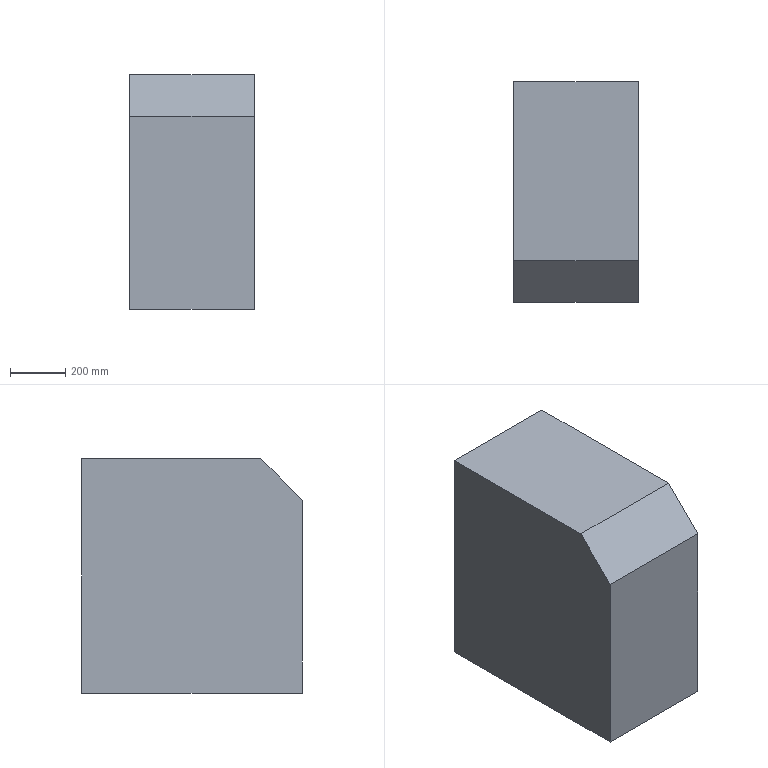Part | NX | features BREP 1 | 1 solid | 7 faces | box 450 x 800 x 850 mm | volume 300937500 mm3 | plane 7
STEP:
#1=CARTESIAN_POINT('',(225.,-250.,850.));
#2=VERTEX_POINT('',#1);
#3=CARTESIAN_POINT('',(225.,400.,850.));
#4=VERTEX_POINT('',#3);
#5=CARTESIAN_POINT('',(225.,-400.,850.));
#6=DIRECTION('',(0.,1.,0.));
#7=VECTOR('',#6,1000.);
#8=LINE('',#5,#7);
#9=EDGE_CURVE('',#2,#4,#8,.T.);
#10=ORIENTED_EDGE('',*,*,#9,.F.);
#11=CARTESIAN_POINT('',(225.,-400.,700.));
#12=VERTEX_POINT('',#11);
#13=CARTESIAN_POINT('',(225.,-250.,850.));
#14=DIRECTION('',(0.,-0.7071,-0.7071));
#15=VECTOR('',#14,1000.);
#16=LINE('',#13,#15);
#17=EDGE_CURVE('',#2,#12,#16,.T.);
#18=ORIENTED_EDGE('',*,*,#17,.T.);
#19=CARTESIAN_POINT('',(225.,-400.,0.));
#20=VERTEX_POINT('',#19);
#21=CARTESIAN_POINT('',(225.,-400.,850.));
#22=DIRECTION('',(0.,0.,-1.));
#23=VECTOR('',#22,1000.);
#24=LINE('',#21,#23);
#25=EDGE_CURVE('',#12,#20,#24,.T.);
#26=ORIENTED_EDGE('',*,*,#25,.T.);
#27=CARTESIAN_POINT('',(225.,400.,0.));
#28=VERTEX_POINT('',#27);
#29=CARTESIAN_POINT('',(225.,-400.,0.));
#30=DIRECTION('',(0.,1.,0.));
#31=VECTOR('',#30,1000.);
#32=LINE('',#29,#31);
#33=EDGE_CURVE('',#20,#28,#32,.T.);
#34=ORIENTED_EDGE('',*,*,#33,.T.);
#35=CARTESIAN_POINT('',(225.,400.,850.));
#36=DIRECTION('',(0.,0.,-1.));
#37=VECTOR('',#36,1000.);
#38=LINE('',#35,#37);
#39=EDGE_CURVE('',#4,#28,#38,.T.);
#40=ORIENTED_EDGE('',*,*,#39,.F.);
#41=EDGE_LOOP('',(#10,#18,#26,#34,#40));
#42=FACE_BOUND('',#41,.T.);
#43=CARTESIAN_POINT('',(225.,-400.,850.));
#44=DIRECTION('',(-1.,0.,0.));
#45=DIRECTION('',(0.,0.,1.));
#46=AXIS2_PLACEMENT_3D('',#43,#44,#45);
#47=PLANE('',#46);
#48=ADVANCED_FACE('',(#42),#47,.F.);
#49=CARTESIAN_POINT('',(-225.,400.,0.));
#50=VERTEX_POINT('',#49);
#51=CARTESIAN_POINT('',(-225.,400.,0.));
#52=DIRECTION('',(-1.,0.,0.));
#53=VECTOR('',#52,1000.);
#54=LINE('',#51,#53);
#55=EDGE_CURVE('',#28,#50,#54,.T.);
#56=ORIENTED_EDGE('',*,*,#55,.T.);
#57=CARTESIAN_POINT('',(-225.,400.,850.));
#58=VERTEX_POINT('',#57);
#59=CARTESIAN_POINT('',(-225.,400.,850.));
#60=DIRECTION('',(0.,0.,-1.));
#61=VECTOR('',#60,1000.);
#62=LINE('',#59,#61);
#63=EDGE_CURVE('',#58,#50,#62,.T.);
#64=ORIENTED_EDGE('',*,*,#63,.F.);
#65=CARTESIAN_POINT('',(-225.,400.,850.));
#66=DIRECTION('',(-1.,0.,0.));
#67=VECTOR('',#66,1000.);
#68=LINE('',#65,#67);
#69=EDGE_CURVE('',#4,#58,#68,.T.);
#70=ORIENTED_EDGE('',*,*,#69,.F.);
#71=ORIENTED_EDGE('',*,*,#39,.T.);
#72=EDGE_LOOP('',(#56,#64,#70,#71));
#73=FACE_BOUND('',#72,.T.);
#74=CARTESIAN_POINT('',(-225.,400.,850.));
#75=DIRECTION('',(0.,-1.,0.));
#76=DIRECTION('',(0.,0.,-1.));
#77=AXIS2_PLACEMENT_3D('',#74,#75,#76);
#78=PLANE('',#77);
#79=ADVANCED_FACE('',(#73),#78,.F.);
#80=CARTESIAN_POINT('',(-225.,-400.,700.));
#81=VERTEX_POINT('',#80);
#82=CARTESIAN_POINT('',(-225.,-400.,0.));
#83=VERTEX_POINT('',#82);
#84=CARTESIAN_POINT('',(-225.,-400.,850.));
#85=DIRECTION('',(0.,0.,-1.));
#86=VECTOR('',#85,1000.);
#87=LINE('',#84,#86);
#88=EDGE_CURVE('',#81,#83,#87,.T.);
#89=ORIENTED_EDGE('',*,*,#88,.F.);
#90=CARTESIAN_POINT('',(-225.,-250.,850.));
#91=VERTEX_POINT('',#90);
#92=CARTESIAN_POINT('',(-225.,-250.,850.));
#93=DIRECTION('',(0.,0.7071,0.7071));
#94=VECTOR('',#93,1000.);
#95=LINE('',#92,#94);
#96=EDGE_CURVE('',#81,#91,#95,.T.);
#97=ORIENTED_EDGE('',*,*,#96,.T.);
#98=CARTESIAN_POINT('',(-225.,-400.,850.));
#99=DIRECTION('',(0.,-1.,0.));
#100=VECTOR('',#99,1000.);
#101=LINE('',#98,#100);
#102=EDGE_CURVE('',#58,#91,#101,.T.);
#103=ORIENTED_EDGE('',*,*,#102,.F.);
#104=ORIENTED_EDGE('',*,*,#63,.T.);
#105=CARTESIAN_POINT('',(-225.,-400.,0.));
#106=DIRECTION('',(0.,-1.,0.));
#107=VECTOR('',#106,1000.);
#108=LINE('',#105,#107);
#109=EDGE_CURVE('',#50,#83,#108,.T.);
#110=ORIENTED_EDGE('',*,*,#109,.T.);
#111=EDGE_LOOP('',(#89,#97,#103,#104,#110));
#112=FACE_BOUND('',#111,.T.);
#113=CARTESIAN_POINT('',(-225.,-400.,850.));
#114=DIRECTION('',(1.,0.,0.));
#115=DIRECTION('',(0.,1.,0.));
#116=AXIS2_PLACEMENT_3D('',#113,#114,#115);
#117=PLANE('',#116);
#118=ADVANCED_FACE('',(#112),#117,.F.);
#119=ORIENTED_EDGE('',*,*,#25,.F.);
#120=CARTESIAN_POINT('',(-225.,-400.,700.));
#121=DIRECTION('',(-1.,0.,0.));
#122=VECTOR('',#121,1000.);
#123=LINE('',#120,#122);
#124=EDGE_CURVE('',#12,#81,#123,.T.);
#125=ORIENTED_EDGE('',*,*,#124,.T.);
#126=ORIENTED_EDGE('',*,*,#88,.T.);
#127=CARTESIAN_POINT('',(-225.,-400.,0.));
#128=DIRECTION('',(1.,0.,0.));
#129=VECTOR('',#128,1000.);
#130=LINE('',#127,#129);
#131=EDGE_CURVE('',#83,#20,#130,.T.);
#132=ORIENTED_EDGE('',*,*,#131,.T.);
#133=EDGE_LOOP('',(#119,#125,#126,#132));
#134=FACE_BOUND('',#133,.T.);
#135=CARTESIAN_POINT('',(-225.,-400.,850.));
#136=DIRECTION('',(0.,1.,0.));
#137=DIRECTION('',(1.,0.,0.));
#138=AXIS2_PLACEMENT_3D('',#135,#136,#137);
#139=PLANE('',#138);
#140=ADVANCED_FACE('',(#134),#139,.F.);
#141=ORIENTED_EDGE('',*,*,#102,.T.);
#142=CARTESIAN_POINT('',(0.,-250.,850.));
#143=DIRECTION('',(1.,0.,0.));
#144=VECTOR('',#143,1000.);
#145=LINE('',#142,#144);
#146=EDGE_CURVE('',#91,#2,#145,.T.);
#147=ORIENTED_EDGE('',*,*,#146,.T.);
#148=ORIENTED_EDGE('',*,*,#9,.T.);
#149=ORIENTED_EDGE('',*,*,#69,.T.);
#150=EDGE_LOOP('',(#141,#147,#148,#149));
#151=FACE_BOUND('',#150,.T.);
#152=CARTESIAN_POINT('',(0.,0.,850.));
#153=DIRECTION('',(0.,0.,-1.));
#154=DIRECTION('',(0.,-1.,0.));
#155=AXIS2_PLACEMENT_3D('',#152,#153,#154);
#156=PLANE('',#155);
#157=ADVANCED_FACE('',(#151),#156,.F.);
#158=ORIENTED_EDGE('',*,*,#33,.F.);
#159=ORIENTED_EDGE('',*,*,#131,.F.);
#160=ORIENTED_EDGE('',*,*,#109,.F.);
#161=ORIENTED_EDGE('',*,*,#55,.F.);
#162=EDGE_LOOP('',(#158,#159,#160,#161));
#163=FACE_BOUND('',#162,.T.);
#164=CARTESIAN_POINT('',(0.,0.,0.));
#165=DIRECTION('',(0.,0.,-1.));
#166=DIRECTION('',(0.,-1.,0.));
#167=AXIS2_PLACEMENT_3D('',#164,#165,#166);
#168=PLANE('',#167);
#169=ADVANCED_FACE('',(#163),#168,.T.);
#170=ORIENTED_EDGE('',*,*,#96,.F.);
#171=ORIENTED_EDGE('',*,*,#124,.F.);
#172=ORIENTED_EDGE('',*,*,#17,.F.);
#173=ORIENTED_EDGE('',*,*,#146,.F.);
#174=EDGE_LOOP('',(#170,#171,#172,#173));
#175=FACE_BOUND('',#174,.T.);
#176=CARTESIAN_POINT('',(0.,-250.,850.));
#177=DIRECTION('',(0.,0.7071,-0.7071));
#178=DIRECTION('',(-1.,0.,0.));
#179=AXIS2_PLACEMENT_3D('',#176,#177,#178);
#180=PLANE('',#179);
#181=ADVANCED_FACE('',(#175),#180,.F.);
#182=CLOSED_SHELL('',(#48,#79,#118,#140,#157,#169,#181));
#183=MANIFOLD_SOLID_BREP('',#182);
#184=(LENGTH_UNIT()NAMED_UNIT(*)SI_UNIT(.MILLI.,.METRE.));
#185=UNCERTAINTY_MEASURE_WITH_UNIT(LENGTH_MEASURE(0.00001),#184,'','');
#186=(NAMED_UNIT(*)PLANE_ANGLE_UNIT()SI_UNIT($,.RADIAN.));
#187=(NAMED_UNIT(*)SI_UNIT($,.STERADIAN.)SOLID_ANGLE_UNIT());
#188=(GEOMETRIC_REPRESENTATION_CONTEXT(3)GLOBAL_UNCERTAINTY_ASSIGNED_CONTEXT((#185))GLOBAL_UNIT_ASSIGNED_CONTEXT((#184,#186,#187))REPRESENTATION_CONTEXT('',''));
#189=ADVANCED_BREP_SHAPE_REPRESENTATION('',(#183),#188);